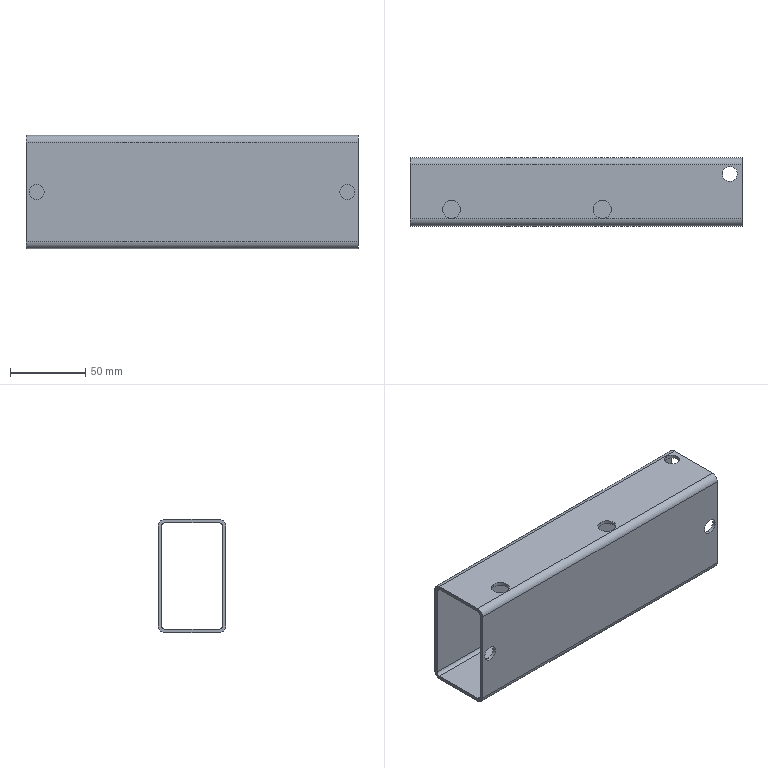Part | STEP file | [07] | 1 solid | 30 faces | box 220 x 45 x 75 mm | volume 112545 mm3 | cylinder 20 | plane 10 | commonest cylinder face diameters 10 x8 4.6 x4 9.2 x4 12 x4
STEP:
#1=CARTESIAN_POINT('',(213.,0.,32.5));
#2=VERTEX_POINT('',#1);
#3=CARTESIAN_POINT('',(213.,0.,42.5));
#4=VERTEX_POINT('',#3);
#5=CARTESIAN_POINT('',(213.,0.,37.5));
#6=DIRECTION('',(0.,1.,0.));
#7=DIRECTION('',(0.,0.,1.));
#8=AXIS2_PLACEMENT_3D('',#5,#6,#7);
#9=CIRCLE('',#8,5.);
#10=EDGE_CURVE('',#2,#4,#9,.T.);
#11=ORIENTED_EDGE('',*,*,#10,.F.);
#12=CARTESIAN_POINT('',(213.,2.3,32.5));
#13=VERTEX_POINT('',#12);
#14=CARTESIAN_POINT('',(213.,0.,32.5));
#15=DIRECTION('',(0.,1.,0.));
#16=VECTOR('',#15,1000.);
#17=LINE('',#14,#16);
#18=EDGE_CURVE('',#2,#13,#17,.T.);
#19=ORIENTED_EDGE('',*,*,#18,.T.);
#20=CARTESIAN_POINT('',(213.,2.3,42.5));
#21=VERTEX_POINT('',#20);
#22=CARTESIAN_POINT('',(213.,2.3,37.5));
#23=DIRECTION('',(0.,-1.,0.));
#24=DIRECTION('',(0.,0.,-1.));
#25=AXIS2_PLACEMENT_3D('',#22,#23,#24);
#26=CIRCLE('',#25,5.);
#27=EDGE_CURVE('',#21,#13,#26,.T.);
#28=ORIENTED_EDGE('',*,*,#27,.F.);
#29=CARTESIAN_POINT('',(213.,0.,42.5));
#30=DIRECTION('',(0.,1.,0.));
#31=VECTOR('',#30,1000.);
#32=LINE('',#29,#31);
#33=EDGE_CURVE('',#4,#21,#32,.T.);
#34=ORIENTED_EDGE('',*,*,#33,.F.);
#35=EDGE_LOOP('',(#11,#19,#28,#34));
#36=FACE_OUTER_BOUND('',#35,.T.);
#37=CARTESIAN_POINT('',(213.,0.,37.5));
#38=DIRECTION('',(0.,1.,0.));
#39=DIRECTION('',(0.,0.,1.));
#40=AXIS2_PLACEMENT_3D('',#37,#38,#39);
#41=CYLINDRICAL_SURFACE('',#40,5.);
#42=ADVANCED_FACE('',(#36),#41,.F.);
#43=CARTESIAN_POINT('',(7.,0.,32.5));
#44=VERTEX_POINT('',#43);
#45=CARTESIAN_POINT('',(7.,0.,42.5));
#46=VERTEX_POINT('',#45);
#47=CARTESIAN_POINT('',(7.,0.,37.5));
#48=DIRECTION('',(0.,1.,0.));
#49=DIRECTION('',(0.,0.,1.));
#50=AXIS2_PLACEMENT_3D('',#47,#48,#49);
#51=CIRCLE('',#50,5.);
#52=EDGE_CURVE('',#44,#46,#51,.T.);
#53=ORIENTED_EDGE('',*,*,#52,.F.);
#54=CARTESIAN_POINT('',(7.,2.3,32.5));
#55=VERTEX_POINT('',#54);
#56=CARTESIAN_POINT('',(7.,0.,32.5));
#57=DIRECTION('',(0.,1.,0.));
#58=VECTOR('',#57,1000.);
#59=LINE('',#56,#58);
#60=EDGE_CURVE('',#44,#55,#59,.T.);
#61=ORIENTED_EDGE('',*,*,#60,.T.);
#62=CARTESIAN_POINT('',(7.,2.3,42.5));
#63=VERTEX_POINT('',#62);
#64=CARTESIAN_POINT('',(7.,2.3,37.5));
#65=DIRECTION('',(0.,-1.,0.));
#66=DIRECTION('',(0.,0.,-1.));
#67=AXIS2_PLACEMENT_3D('',#64,#65,#66);
#68=CIRCLE('',#67,5.);
#69=EDGE_CURVE('',#63,#55,#68,.T.);
#70=ORIENTED_EDGE('',*,*,#69,.F.);
#71=CARTESIAN_POINT('',(7.,0.,42.5));
#72=DIRECTION('',(0.,1.,0.));
#73=VECTOR('',#72,1000.);
#74=LINE('',#71,#73);
#75=EDGE_CURVE('',#46,#63,#74,.T.);
#76=ORIENTED_EDGE('',*,*,#75,.F.);
#77=EDGE_LOOP('',(#53,#61,#70,#76));
#78=FACE_OUTER_BOUND('',#77,.T.);
#79=CARTESIAN_POINT('',(7.,0.,37.5));
#80=DIRECTION('',(0.,1.,0.));
#81=DIRECTION('',(0.,0.,1.));
#82=AXIS2_PLACEMENT_3D('',#79,#80,#81);
#83=CYLINDRICAL_SURFACE('',#82,5.);
#84=ADVANCED_FACE('',(#78),#83,.F.);
#85=CARTESIAN_POINT('',(212.,29.5,2.3));
#86=VERTEX_POINT('',#85);
#87=CARTESIAN_POINT('',(212.,39.5,2.3));
#88=VERTEX_POINT('',#87);
#89=CARTESIAN_POINT('',(212.,34.5,2.3));
#90=DIRECTION('',(0.,0.,-1.));
#91=DIRECTION('',(0.,1.,0.));
#92=AXIS2_PLACEMENT_3D('',#89,#90,#91);
#93=CIRCLE('',#92,5.);
#94=EDGE_CURVE('',#86,#88,#93,.T.);
#95=ORIENTED_EDGE('',*,*,#94,.F.);
#96=CARTESIAN_POINT('',(212.,29.5,0.));
#97=VERTEX_POINT('',#96);
#98=CARTESIAN_POINT('',(212.,29.5,2.3));
#99=DIRECTION('',(0.,0.,-1.));
#100=VECTOR('',#99,1000.);
#101=LINE('',#98,#100);
#102=EDGE_CURVE('',#86,#97,#101,.T.);
#103=ORIENTED_EDGE('',*,*,#102,.T.);
#104=CARTESIAN_POINT('',(212.,39.5,0.));
#105=VERTEX_POINT('',#104);
#106=CARTESIAN_POINT('',(212.,34.5,0.));
#107=DIRECTION('',(0.,0.,1.));
#108=DIRECTION('',(0.,-1.,0.));
#109=AXIS2_PLACEMENT_3D('',#106,#107,#108);
#110=CIRCLE('',#109,5.);
#111=EDGE_CURVE('',#105,#97,#110,.T.);
#112=ORIENTED_EDGE('',*,*,#111,.F.);
#113=CARTESIAN_POINT('',(212.,39.5,2.3));
#114=DIRECTION('',(0.,0.,-1.));
#115=VECTOR('',#114,1000.);
#116=LINE('',#113,#115);
#117=EDGE_CURVE('',#88,#105,#116,.T.);
#118=ORIENTED_EDGE('',*,*,#117,.F.);
#119=EDGE_LOOP('',(#95,#103,#112,#118));
#120=FACE_OUTER_BOUND('',#119,.T.);
#121=CARTESIAN_POINT('',(212.,34.5,2.3));
#122=DIRECTION('',(0.,0.,-1.));
#123=DIRECTION('',(0.,1.,0.));
#124=AXIS2_PLACEMENT_3D('',#121,#122,#123);
#125=CYLINDRICAL_SURFACE('',#124,5.);
#126=ADVANCED_FACE('',(#120),#125,.F.);
#127=CARTESIAN_POINT('',(127.5,5.,75.));
#128=VERTEX_POINT('',#127);
#129=CARTESIAN_POINT('',(127.5,17.,75.));
#130=VERTEX_POINT('',#129);
#131=CARTESIAN_POINT('',(127.5,11.,75.));
#132=DIRECTION('',(0.,0.,-1.));
#133=DIRECTION('',(0.,1.,0.));
#134=AXIS2_PLACEMENT_3D('',#131,#132,#133);
#135=CIRCLE('',#134,6.);
#136=EDGE_CURVE('',#128,#130,#135,.T.);
#137=ORIENTED_EDGE('',*,*,#136,.F.);
#138=CARTESIAN_POINT('',(127.5,5.,72.7));
#139=VERTEX_POINT('',#138);
#140=CARTESIAN_POINT('',(127.5,5.,75.));
#141=DIRECTION('',(0.,0.,-1.));
#142=VECTOR('',#141,1000.);
#143=LINE('',#140,#142);
#144=EDGE_CURVE('',#128,#139,#143,.T.);
#145=ORIENTED_EDGE('',*,*,#144,.T.);
#146=CARTESIAN_POINT('',(127.5,17.,72.7));
#147=VERTEX_POINT('',#146);
#148=CARTESIAN_POINT('',(127.5,11.,72.7));
#149=DIRECTION('',(0.,0.,1.));
#150=DIRECTION('',(0.,-1.,0.));
#151=AXIS2_PLACEMENT_3D('',#148,#149,#150);
#152=CIRCLE('',#151,6.);
#153=EDGE_CURVE('',#147,#139,#152,.T.);
#154=ORIENTED_EDGE('',*,*,#153,.F.);
#155=CARTESIAN_POINT('',(127.5,17.,75.));
#156=DIRECTION('',(0.,0.,-1.));
#157=VECTOR('',#156,1000.);
#158=LINE('',#155,#157);
#159=EDGE_CURVE('',#130,#147,#158,.T.);
#160=ORIENTED_EDGE('',*,*,#159,.F.);
#161=EDGE_LOOP('',(#137,#145,#154,#160));
#162=FACE_OUTER_BOUND('',#161,.T.);
#163=CARTESIAN_POINT('',(127.5,11.,75.));
#164=DIRECTION('',(0.,0.,-1.));
#165=DIRECTION('',(0.,1.,0.));
#166=AXIS2_PLACEMENT_3D('',#163,#164,#165);
#167=CYLINDRICAL_SURFACE('',#166,6.);
#168=ADVANCED_FACE('',(#162),#167,.F.);
#169=CARTESIAN_POINT('',(212.,29.5,75.));
#170=VERTEX_POINT('',#169);
#171=CARTESIAN_POINT('',(212.,39.5,75.));
#172=VERTEX_POINT('',#171);
#173=CARTESIAN_POINT('',(212.,34.5,75.));
#174=DIRECTION('',(0.,0.,-1.));
#175=DIRECTION('',(0.,1.,0.));
#176=AXIS2_PLACEMENT_3D('',#173,#174,#175);
#177=CIRCLE('',#176,5.);
#178=EDGE_CURVE('',#170,#172,#177,.T.);
#179=ORIENTED_EDGE('',*,*,#178,.F.);
#180=CARTESIAN_POINT('',(212.,29.5,72.7));
#181=VERTEX_POINT('',#180);
#182=CARTESIAN_POINT('',(212.,29.5,75.));
#183=DIRECTION('',(0.,0.,-1.));
#184=VECTOR('',#183,1000.);
#185=LINE('',#182,#184);
#186=EDGE_CURVE('',#170,#181,#185,.T.);
#187=ORIENTED_EDGE('',*,*,#186,.T.);
#188=CARTESIAN_POINT('',(212.,39.5,72.7));
#189=VERTEX_POINT('',#188);
#190=CARTESIAN_POINT('',(212.,34.5,72.7));
#191=DIRECTION('',(0.,0.,1.));
#192=DIRECTION('',(0.,-1.,0.));
#193=AXIS2_PLACEMENT_3D('',#190,#191,#192);
#194=CIRCLE('',#193,5.);
#195=EDGE_CURVE('',#189,#181,#194,.T.);
#196=ORIENTED_EDGE('',*,*,#195,.F.);
#197=CARTESIAN_POINT('',(212.,39.5,75.));
#198=DIRECTION('',(0.,0.,-1.));
#199=VECTOR('',#198,1000.);
#200=LINE('',#197,#199);
#201=EDGE_CURVE('',#172,#189,#200,.T.);
#202=ORIENTED_EDGE('',*,*,#201,.F.);
#203=EDGE_LOOP('',(#179,#187,#196,#202));
#204=FACE_OUTER_BOUND('',#203,.T.);
#205=CARTESIAN_POINT('',(212.,34.5,75.));
#206=DIRECTION('',(0.,0.,-1.));
#207=DIRECTION('',(0.,1.,0.));
#208=AXIS2_PLACEMENT_3D('',#205,#206,#207);
#209=CYLINDRICAL_SURFACE('',#208,5.);
#210=ADVANCED_FACE('',(#204),#209,.F.);
#211=CARTESIAN_POINT('',(27.5,5.,75.));
#212=VERTEX_POINT('',#211);
#213=CARTESIAN_POINT('',(27.5,17.,75.));
#214=VERTEX_POINT('',#213);
#215=CARTESIAN_POINT('',(27.5,11.,75.));
#216=DIRECTION('',(0.,0.,-1.));
#217=DIRECTION('',(0.,1.,0.));
#218=AXIS2_PLACEMENT_3D('',#215,#216,#217);
#219=CIRCLE('',#218,6.);
#220=EDGE_CURVE('',#212,#214,#219,.T.);
#221=ORIENTED_EDGE('',*,*,#220,.F.);
#222=CARTESIAN_POINT('',(27.5,5.,72.7));
#223=VERTEX_POINT('',#222);
#224=CARTESIAN_POINT('',(27.5,5.,75.));
#225=DIRECTION('',(0.,0.,-1.));
#226=VECTOR('',#225,1000.);
#227=LINE('',#224,#226);
#228=EDGE_CURVE('',#212,#223,#227,.T.);
#229=ORIENTED_EDGE('',*,*,#228,.T.);
#230=CARTESIAN_POINT('',(27.5,17.,72.7));
#231=VERTEX_POINT('',#230);
#232=CARTESIAN_POINT('',(27.5,11.,72.7));
#233=DIRECTION('',(0.,0.,1.));
#234=DIRECTION('',(0.,-1.,0.));
#235=AXIS2_PLACEMENT_3D('',#232,#233,#234);
#236=CIRCLE('',#235,6.);
#237=EDGE_CURVE('',#231,#223,#236,.T.);
#238=ORIENTED_EDGE('',*,*,#237,.F.);
#239=CARTESIAN_POINT('',(27.5,17.,75.));
#240=DIRECTION('',(0.,0.,-1.));
#241=VECTOR('',#240,1000.);
#242=LINE('',#239,#241);
#243=EDGE_CURVE('',#214,#231,#242,.T.);
#244=ORIENTED_EDGE('',*,*,#243,.F.);
#245=EDGE_LOOP('',(#221,#229,#238,#244));
#246=FACE_OUTER_BOUND('',#245,.T.);
#247=CARTESIAN_POINT('',(27.5,11.,75.));
#248=DIRECTION('',(0.,0.,-1.));
#249=DIRECTION('',(0.,1.,0.));
#250=AXIS2_PLACEMENT_3D('',#247,#248,#249);
#251=CYLINDRICAL_SURFACE('',#250,6.);
#252=ADVANCED_FACE('',(#246),#251,.F.);
#253=CARTESIAN_POINT('',(213.,0.,37.5));
#254=DIRECTION('',(0.,1.,0.));
#255=DIRECTION('',(0.,0.,1.));
#256=AXIS2_PLACEMENT_3D('',#253,#254,#255);
#257=CIRCLE('',#256,5.);
#258=EDGE_CURVE('',#4,#2,#257,.T.);
#259=ORIENTED_EDGE('',*,*,#258,.T.);
#260=ORIENTED_EDGE('',*,*,#10,.T.);
#261=EDGE_LOOP('',(#259,#260));
#262=FACE_BOUND('',#261,.T.);
#263=CARTESIAN_POINT('',(7.,0.,37.5));
#264=DIRECTION('',(0.,1.,0.));
#265=DIRECTION('',(0.,0.,1.));
#266=AXIS2_PLACEMENT_3D('',#263,#264,#265);
#267=CIRCLE('',#266,5.);
#268=EDGE_CURVE('',#46,#44,#267,.T.);
#269=ORIENTED_EDGE('',*,*,#268,.T.);
#270=ORIENTED_EDGE('',*,*,#52,.T.);
#271=EDGE_LOOP('',(#269,#270));
#272=FACE_BOUND('',#271,.T.);
#273=CARTESIAN_POINT('',(220.,0.,70.4));
#274=VERTEX_POINT('',#273);
#275=CARTESIAN_POINT('',(220.,0.,4.6));
#276=VERTEX_POINT('',#275);
#277=CARTESIAN_POINT('',(220.,0.,70.4));
#278=DIRECTION('',(0.,0.,-1.));
#279=VECTOR('',#278,1000.);
#280=LINE('',#277,#279);
#281=EDGE_CURVE('',#274,#276,#280,.T.);
#282=ORIENTED_EDGE('',*,*,#281,.F.);
#283=CARTESIAN_POINT('',(0.,0.,70.4));
#284=VERTEX_POINT('',#283);
#285=CARTESIAN_POINT('',(0.,0.,70.4));
#286=DIRECTION('',(1.,0.,0.));
#287=VECTOR('',#286,1000.);
#288=LINE('',#285,#287);
#289=EDGE_CURVE('',#284,#274,#288,.T.);
#290=ORIENTED_EDGE('',*,*,#289,.F.);
#291=CARTESIAN_POINT('',(0.,0.,4.6));
#292=VERTEX_POINT('',#291);
#293=CARTESIAN_POINT('',(0.,0.,70.4));
#294=DIRECTION('',(0.,0.,-1.));
#295=VECTOR('',#294,1000.);
#296=LINE('',#293,#295);
#297=EDGE_CURVE('',#284,#292,#296,.T.);
#298=ORIENTED_EDGE('',*,*,#297,.T.);
#299=CARTESIAN_POINT('',(0.,0.,4.6));
#300=DIRECTION('',(1.,0.,0.));
#301=VECTOR('',#300,1000.);
#302=LINE('',#299,#301);
#303=EDGE_CURVE('',#292,#276,#302,.T.);
#304=ORIENTED_EDGE('',*,*,#303,.T.);
#305=EDGE_LOOP('',(#282,#290,#298,#304));
#306=FACE_OUTER_BOUND('',#305,.T.);
#307=CARTESIAN_POINT('',(0.,0.,70.4));
#308=DIRECTION('',(0.,-1.,0.));
#309=DIRECTION('',(0.,0.,-1.));
#310=AXIS2_PLACEMENT_3D('',#307,#308,#309);
#311=PLANE('',#310);
#312=ADVANCED_FACE('',(#262,#272,#306),#311,.T.);
#313=CARTESIAN_POINT('',(220.,4.6,0.));
#314=VERTEX_POINT('',#313);
#315=CARTESIAN_POINT('',(220.,4.6,4.6));
#316=DIRECTION('',(1.,0.,0.));
#317=DIRECTION('',(0.,-1.,0.));
#318=AXIS2_PLACEMENT_3D('',#315,#316,#317);
#319=CIRCLE('',#318,4.6);
#320=EDGE_CURVE('',#276,#314,#319,.T.);
#321=ORIENTED_EDGE('',*,*,#320,.F.);
#322=ORIENTED_EDGE('',*,*,#303,.F.);
#323=CARTESIAN_POINT('',(0.,4.6,0.));
#324=VERTEX_POINT('',#323);
#325=CARTESIAN_POINT('',(0.,4.6,4.6));
#326=DIRECTION('',(1.,0.,0.));
#327=DIRECTION('',(0.,-1.,0.));
#328=AXIS2_PLACEMENT_3D('',#325,#326,#327);
#329=CIRCLE('',#328,4.6);
#330=EDGE_CURVE('',#292,#324,#329,.T.);
#331=ORIENTED_EDGE('',*,*,#330,.T.);
#332=CARTESIAN_POINT('',(0.,4.6,0.));
#333=DIRECTION('',(1.,0.,0.));
#334=VECTOR('',#333,1000.);
#335=LINE('',#332,#334);
#336=EDGE_CURVE('',#324,#314,#335,.T.);
#337=ORIENTED_EDGE('',*,*,#336,.T.);
#338=EDGE_LOOP('',(#321,#322,#331,#337));
#339=FACE_OUTER_BOUND('',#338,.T.);
#340=CARTESIAN_POINT('',(0.,4.6,4.6));
#341=DIRECTION('',(1.,0.,0.));
#342=DIRECTION('',(0.,-1.,0.));
#343=AXIS2_PLACEMENT_3D('',#340,#341,#342);
#344=CYLINDRICAL_SURFACE('',#343,4.6);
#345=ADVANCED_FACE('',(#339),#344,.T.);
#346=ORIENTED_EDGE('',*,*,#111,.T.);
#347=CARTESIAN_POINT('',(212.,34.5,0.));
#348=DIRECTION('',(0.,0.,1.));
#349=DIRECTION('',(0.,-1.,0.));
#350=AXIS2_PLACEMENT_3D('',#347,#348,#349);
#351=CIRCLE('',#350,5.);
#352=EDGE_CURVE('',#97,#105,#351,.T.);
#353=ORIENTED_EDGE('',*,*,#352,.T.);
#354=EDGE_LOOP('',(#346,#353));
#355=FACE_BOUND('',#354,.T.);
#356=CARTESIAN_POINT('',(220.,40.4,0.));
#357=VERTEX_POINT('',#356);
#358=CARTESIAN_POINT('',(220.,4.6,0.));
#359=DIRECTION('',(0.,1.,0.));
#360=VECTOR('',#359,1000.);
#361=LINE('',#358,#360);
#362=EDGE_CURVE('',#314,#357,#361,.T.);
#363=ORIENTED_EDGE('',*,*,#362,.F.);
#364=ORIENTED_EDGE('',*,*,#336,.F.);
#365=CARTESIAN_POINT('',(0.,40.4,0.));
#366=VERTEX_POINT('',#365);
#367=CARTESIAN_POINT('',(0.,4.6,0.));
#368=DIRECTION('',(0.,1.,0.));
#369=VECTOR('',#368,1000.);
#370=LINE('',#367,#369);
#371=EDGE_CURVE('',#324,#366,#370,.T.);
#372=ORIENTED_EDGE('',*,*,#371,.T.);
#373=CARTESIAN_POINT('',(0.,40.4,0.));
#374=DIRECTION('',(1.,0.,0.));
#375=VECTOR('',#374,1000.);
#376=LINE('',#373,#375);
#377=EDGE_CURVE('',#366,#357,#376,.T.);
#378=ORIENTED_EDGE('',*,*,#377,.T.);
#379=EDGE_LOOP('',(#363,#364,#372,#378));
#380=FACE_OUTER_BOUND('',#379,.T.);
#381=CARTESIAN_POINT('',(0.,4.6,0.));
#382=DIRECTION('',(0.,0.,-1.));
#383=DIRECTION('',(0.,1.,0.));
#384=AXIS2_PLACEMENT_3D('',#381,#382,#383);
#385=PLANE('',#384);
#386=ADVANCED_FACE('',(#355,#380),#385,.T.);
#387=CARTESIAN_POINT('',(220.,45.,4.6));
#388=VERTEX_POINT('',#387);
#389=CARTESIAN_POINT('',(220.,40.4,4.6));
#390=DIRECTION('',(1.,0.,0.));
#391=DIRECTION('',(0.,-1.,0.));
#392=AXIS2_PLACEMENT_3D('',#389,#390,#391);
#393=CIRCLE('',#392,4.6);
#394=EDGE_CURVE('',#357,#388,#393,.T.);
#395=ORIENTED_EDGE('',*,*,#394,.F.);
#396=ORIENTED_EDGE('',*,*,#377,.F.);
#397=CARTESIAN_POINT('',(0.,45.,4.6));
#398=VERTEX_POINT('',#397);
#399=CARTESIAN_POINT('',(0.,40.4,4.6));
#400=DIRECTION('',(1.,0.,0.));
#401=DIRECTION('',(0.,-1.,0.));
#402=AXIS2_PLACEMENT_3D('',#399,#400,#401);
#403=CIRCLE('',#402,4.6);
#404=EDGE_CURVE('',#366,#398,#403,.T.);
#405=ORIENTED_EDGE('',*,*,#404,.T.);
#406=CARTESIAN_POINT('',(0.,45.,4.6));
#407=DIRECTION('',(1.,0.,0.));
#408=VECTOR('',#407,1000.);
#409=LINE('',#406,#408);
#410=EDGE_CURVE('',#398,#388,#409,.T.);
#411=ORIENTED_EDGE('',*,*,#410,.T.);
#412=EDGE_LOOP('',(#395,#396,#405,#411));
#413=FACE_OUTER_BOUND('',#412,.T.);
#414=CARTESIAN_POINT('',(0.,40.4,4.6));
#415=DIRECTION('',(1.,0.,0.));
#416=DIRECTION('',(0.,-1.,0.));
#417=AXIS2_PLACEMENT_3D('',#414,#415,#416);
#418=CYLINDRICAL_SURFACE('',#417,4.6);
#419=ADVANCED_FACE('',(#413),#418,.T.);
#420=CARTESIAN_POINT('',(220.,45.,70.4));
#421=VERTEX_POINT('',#420);
#422=CARTESIAN_POINT('',(220.,45.,4.6));
#423=DIRECTION('',(0.,0.,1.));
#424=VECTOR('',#423,1000.);
#425=LINE('',#422,#424);
#426=EDGE_CURVE('',#388,#421,#425,.T.);
#427=ORIENTED_EDGE('',*,*,#426,.F.);
#428=ORIENTED_EDGE('',*,*,#410,.F.);
#429=CARTESIAN_POINT('',(0.,45.,70.4));
#430=VERTEX_POINT('',#429);
#431=CARTESIAN_POINT('',(0.,45.,4.6));
#432=DIRECTION('',(0.,0.,1.));
#433=VECTOR('',#432,1000.);
#434=LINE('',#431,#433);
#435=EDGE_CURVE('',#398,#430,#434,.T.);
#436=ORIENTED_EDGE('',*,*,#435,.T.);
#437=CARTESIAN_POINT('',(0.,45.,70.4));
#438=DIRECTION('',(1.,0.,0.));
#439=VECTOR('',#438,1000.);
#440=LINE('',#437,#439);
#441=EDGE_CURVE('',#430,#421,#440,.T.);
#442=ORIENTED_EDGE('',*,*,#441,.T.);
#443=EDGE_LOOP('',(#427,#428,#436,#442));
#444=FACE_OUTER_BOUND('',#443,.T.);
#445=CARTESIAN_POINT('',(0.,45.,4.6));
#446=DIRECTION('',(0.,1.,0.));
#447=DIRECTION('',(0.,0.,1.));
#448=AXIS2_PLACEMENT_3D('',#445,#446,#447);
#449=PLANE('',#448);
#450=ADVANCED_FACE('',(#444),#449,.T.);
#451=CARTESIAN_POINT('',(220.,40.4,75.));
#452=VERTEX_POINT('',#451);
#453=CARTESIAN_POINT('',(220.,40.4,70.4));
#454=DIRECTION('',(1.,0.,0.));
#455=DIRECTION('',(0.,-1.,0.));
#456=AXIS2_PLACEMENT_3D('',#453,#454,#455);
#457=CIRCLE('',#456,4.6);
#458=EDGE_CURVE('',#421,#452,#457,.T.);
#459=ORIENTED_EDGE('',*,*,#458,.F.);
#460=ORIENTED_EDGE('',*,*,#441,.F.);
#461=CARTESIAN_POINT('',(0.,40.4,75.));
#462=VERTEX_POINT('',#461);
#463=CARTESIAN_POINT('',(0.,40.4,70.4));
#464=DIRECTION('',(1.,0.,0.));
#465=DIRECTION('',(0.,-1.,0.));
#466=AXIS2_PLACEMENT_3D('',#463,#464,#465);
#467=CIRCLE('',#466,4.6);
#468=EDGE_CURVE('',#430,#462,#467,.T.);
#469=ORIENTED_EDGE('',*,*,#468,.T.);
#470=CARTESIAN_POINT('',(0.,40.4,75.));
#471=DIRECTION('',(1.,0.,0.));
#472=VECTOR('',#471,1000.);
#473=LINE('',#470,#472);
#474=EDGE_CURVE('',#462,#452,#473,.T.);
#475=ORIENTED_EDGE('',*,*,#474,.T.);
#476=EDGE_LOOP('',(#459,#460,#469,#475));
#477=FACE_OUTER_BOUND('',#476,.T.);
#478=CARTESIAN_POINT('',(0.,40.4,70.4));
#479=DIRECTION('',(1.,0.,0.));
#480=DIRECTION('',(0.,-1.,0.));
#481=AXIS2_PLACEMENT_3D('',#478,#479,#480);
#482=CYLINDRICAL_SURFACE('',#481,4.6);
#483=ADVANCED_FACE('',(#477),#482,.T.);
#484=CARTESIAN_POINT('',(127.5,11.,75.));
#485=DIRECTION('',(0.,0.,-1.));
#486=DIRECTION('',(0.,1.,0.));
#487=AXIS2_PLACEMENT_3D('',#484,#485,#486);
#488=CIRCLE('',#487,6.);
#489=EDGE_CURVE('',#130,#128,#488,.T.);
#490=ORIENTED_EDGE('',*,*,#489,.T.);
#491=ORIENTED_EDGE('',*,*,#136,.T.);
#492=EDGE_LOOP('',(#490,#491));
#493=FACE_BOUND('',#492,.T.);
#494=CARTESIAN_POINT('',(212.,34.5,75.));
#495=DIRECTION('',(0.,0.,-1.));
#496=DIRECTION('',(0.,1.,0.));
#497=AXIS2_PLACEMENT_3D('',#494,#495,#496);
#498=CIRCLE('',#497,5.);
#499=EDGE_CURVE('',#172,#170,#498,.T.);
#500=ORIENTED_EDGE('',*,*,#499,.T.);
#501=ORIENTED_EDGE('',*,*,#178,.T.);
#502=EDGE_LOOP('',(#500,#501));
#503=FACE_BOUND('',#502,.T.);
#504=CARTESIAN_POINT('',(27.5,11.,75.));
#505=DIRECTION('',(0.,0.,-1.));
#506=DIRECTION('',(0.,1.,0.));
#507=AXIS2_PLACEMENT_3D('',#504,#505,#506);
#508=CIRCLE('',#507,6.);
#509=EDGE_CURVE('',#214,#212,#508,.T.);
#510=ORIENTED_EDGE('',*,*,#509,.T.);
#511=ORIENTED_EDGE('',*,*,#220,.T.);
#512=EDGE_LOOP('',(#510,#511));
#513=FACE_BOUND('',#512,.T.);
#514=CARTESIAN_POINT('',(220.,4.6,75.));
#515=VERTEX_POINT('',#514);
#516=CARTESIAN_POINT('',(220.,40.4,75.));
#517=DIRECTION('',(0.,-1.,0.));
#518=VECTOR('',#517,1000.);
#519=LINE('',#516,#518);
#520=EDGE_CURVE('',#452,#515,#519,.T.);
#521=ORIENTED_EDGE('',*,*,#520,.F.);
#522=ORIENTED_EDGE('',*,*,#474,.F.);
#523=CARTESIAN_POINT('',(0.,4.6,75.));
#524=VERTEX_POINT('',#523);
#525=CARTESIAN_POINT('',(0.,40.4,75.));
#526=DIRECTION('',(0.,-1.,0.));
#527=VECTOR('',#526,1000.);
#528=LINE('',#525,#527);
#529=EDGE_CURVE('',#462,#524,#528,.T.);
#530=ORIENTED_EDGE('',*,*,#529,.T.);
#531=CARTESIAN_POINT('',(0.,4.6,75.));
#532=DIRECTION('',(1.,0.,0.));
#533=VECTOR('',#532,1000.);
#534=LINE('',#531,#533);
#535=EDGE_CURVE('',#524,#515,#534,.T.);
#536=ORIENTED_EDGE('',*,*,#535,.T.);
#537=EDGE_LOOP('',(#521,#522,#530,#536));
#538=FACE_OUTER_BOUND('',#537,.T.);
#539=CARTESIAN_POINT('',(0.,40.4,75.));
#540=DIRECTION('',(0.,0.,1.));
#541=DIRECTION('',(-1.,0.,0.));
#542=AXIS2_PLACEMENT_3D('',#539,#540,#541);
#543=PLANE('',#542);
#544=ADVANCED_FACE('',(#493,#503,#513,#538),#543,.T.);
#545=CARTESIAN_POINT('',(220.,4.6,70.4));
#546=DIRECTION('',(1.,0.,0.));
#547=DIRECTION('',(0.,-1.,0.));
#548=AXIS2_PLACEMENT_3D('',#545,#546,#547);
#549=CIRCLE('',#548,4.6);
#550=EDGE_CURVE('',#515,#274,#549,.T.);
#551=ORIENTED_EDGE('',*,*,#550,.F.);
#552=ORIENTED_EDGE('',*,*,#535,.F.);
#553=CARTESIAN_POINT('',(0.,4.6,70.4));
#554=DIRECTION('',(1.,0.,0.));
#555=DIRECTION('',(0.,-1.,0.));
#556=AXIS2_PLACEMENT_3D('',#553,#554,#555);
#557=CIRCLE('',#556,4.6);
#558=EDGE_CURVE('',#524,#284,#557,.T.);
#559=ORIENTED_EDGE('',*,*,#558,.T.);
#560=ORIENTED_EDGE('',*,*,#289,.T.);
#561=EDGE_LOOP('',(#551,#552,#559,#560));
#562=FACE_OUTER_BOUND('',#561,.T.);
#563=CARTESIAN_POINT('',(0.,4.6,70.4));
#564=DIRECTION('',(1.,0.,0.));
#565=DIRECTION('',(0.,-1.,0.));
#566=AXIS2_PLACEMENT_3D('',#563,#564,#565);
#567=CYLINDRICAL_SURFACE('',#566,4.6);
#568=ADVANCED_FACE('',(#562),#567,.T.);
#569=CARTESIAN_POINT('',(0.,40.4,72.7));
#570=VERTEX_POINT('',#569);
#571=CARTESIAN_POINT('',(0.,4.6,72.7));
#572=VERTEX_POINT('',#571);
#573=CARTESIAN_POINT('',(0.,40.4,72.7));
#574=DIRECTION('',(0.,-1.,0.));
#575=VECTOR('',#574,1000.);
#576=LINE('',#573,#575);
#577=EDGE_CURVE('',#570,#572,#576,.T.);
#578=ORIENTED_EDGE('',*,*,#577,.T.);
#579=CARTESIAN_POINT('',(0.,2.3,70.4));
#580=VERTEX_POINT('',#579);
#581=CARTESIAN_POINT('',(0.,4.6,70.4));
#582=DIRECTION('',(1.,0.,0.));
#583=DIRECTION('',(0.,0.,1.));
#584=AXIS2_PLACEMENT_3D('',#581,#582,#583);
#585=CIRCLE('',#584,2.3);
#586=EDGE_CURVE('',#572,#580,#585,.T.);
#587=ORIENTED_EDGE('',*,*,#586,.T.);
#588=CARTESIAN_POINT('',(0.,2.3,4.6));
#589=VERTEX_POINT('',#588);
#590=CARTESIAN_POINT('',(0.,2.3,70.4));
#591=DIRECTION('',(0.,0.,-1.));
#592=VECTOR('',#591,1000.);
#593=LINE('',#590,#592);
#594=EDGE_CURVE('',#580,#589,#593,.T.);
#595=ORIENTED_EDGE('',*,*,#594,.T.);
#596=CARTESIAN_POINT('',(0.,4.6,2.3));
#597=VERTEX_POINT('',#596);
#598=CARTESIAN_POINT('',(0.,4.6,4.6));
#599=DIRECTION('',(1.,0.,0.));
#600=DIRECTION('',(0.,0.,1.));
#601=AXIS2_PLACEMENT_3D('',#598,#599,#600);
#602=CIRCLE('',#601,2.3);
#603=EDGE_CURVE('',#589,#597,#602,.T.);
#604=ORIENTED_EDGE('',*,*,#603,.T.);
#605=CARTESIAN_POINT('',(0.,40.4,2.3));
#606=VERTEX_POINT('',#605);
#607=CARTESIAN_POINT('',(0.,4.6,2.3));
#608=DIRECTION('',(0.,1.,0.));
#609=VECTOR('',#608,1000.);
#610=LINE('',#607,#609);
#611=EDGE_CURVE('',#597,#606,#610,.T.);
#612=ORIENTED_EDGE('',*,*,#611,.T.);
#613=CARTESIAN_POINT('',(0.,42.7,4.6));
#614=VERTEX_POINT('',#613);
#615=CARTESIAN_POINT('',(0.,40.4,4.6));
#616=DIRECTION('',(1.,0.,0.));
#617=DIRECTION('',(0.,0.,1.));
#618=AXIS2_PLACEMENT_3D('',#615,#616,#617);
#619=CIRCLE('',#618,2.3);
#620=EDGE_CURVE('',#606,#614,#619,.T.);
#621=ORIENTED_EDGE('',*,*,#620,.T.);
#622=CARTESIAN_POINT('',(0.,42.7,70.4));
#623=VERTEX_POINT('',#622);
#624=CARTESIAN_POINT('',(0.,42.7,4.6));
#625=DIRECTION('',(0.,0.,1.));
#626=VECTOR('',#625,1000.);
#627=LINE('',#624,#626);
#628=EDGE_CURVE('',#614,#623,#627,.T.);
#629=ORIENTED_EDGE('',*,*,#628,.T.);
#630=CARTESIAN_POINT('',(0.,40.4,70.4));
#631=DIRECTION('',(1.,0.,0.));
#632=DIRECTION('',(0.,0.,1.));
#633=AXIS2_PLACEMENT_3D('',#630,#631,#632);
#634=CIRCLE('',#633,2.3);
#635=EDGE_CURVE('',#623,#570,#634,.T.);
#636=ORIENTED_EDGE('',*,*,#635,.T.);
#637=EDGE_LOOP('',(#578,#587,#595,#604,#612,#621,#629,#636));
#638=FACE_BOUND('',#637,.T.);
#639=ORIENTED_EDGE('',*,*,#297,.F.);
#640=ORIENTED_EDGE('',*,*,#558,.F.);
#641=ORIENTED_EDGE('',*,*,#529,.F.);
#642=ORIENTED_EDGE('',*,*,#468,.F.);
#643=ORIENTED_EDGE('',*,*,#435,.F.);
#644=ORIENTED_EDGE('',*,*,#404,.F.);
#645=ORIENTED_EDGE('',*,*,#371,.F.);
#646=ORIENTED_EDGE('',*,*,#330,.F.);
#647=EDGE_LOOP('',(#639,#640,#641,#642,#643,#644,#645,#646));
#648=FACE_OUTER_BOUND('',#647,.T.);
#649=CARTESIAN_POINT('',(0.,4.6,4.6));
#650=DIRECTION('',(1.,0.,0.));
#651=DIRECTION('',(0.,-1.,0.));
#652=AXIS2_PLACEMENT_3D('',#649,#650,#651);
#653=PLANE('',#652);
#654=ADVANCED_FACE('',(#638,#648),#653,.F.);
#655=CARTESIAN_POINT('',(220.,4.6,72.7));
#656=VERTEX_POINT('',#655);
#657=CARTESIAN_POINT('',(220.,2.3,70.4));
#658=VERTEX_POINT('',#657);
#659=CARTESIAN_POINT('',(220.,4.6,70.4));
#660=DIRECTION('',(1.,0.,0.));
#661=DIRECTION('',(0.,0.,1.));
#662=AXIS2_PLACEMENT_3D('',#659,#660,#661);
#663=CIRCLE('',#662,2.3);
#664=EDGE_CURVE('',#656,#658,#663,.T.);
#665=ORIENTED_EDGE('',*,*,#664,.F.);
#666=CARTESIAN_POINT('',(220.,40.4,72.7));
#667=VERTEX_POINT('',#666);
#668=CARTESIAN_POINT('',(220.,40.4,72.7));
#669=DIRECTION('',(0.,-1.,0.));
#670=VECTOR('',#669,1000.);
#671=LINE('',#668,#670);
#672=EDGE_CURVE('',#667,#656,#671,.T.);
#673=ORIENTED_EDGE('',*,*,#672,.F.);
#674=CARTESIAN_POINT('',(220.,42.7,70.4));
#675=VERTEX_POINT('',#674);
#676=CARTESIAN_POINT('',(220.,40.4,70.4));
#677=DIRECTION('',(1.,0.,0.));
#678=DIRECTION('',(0.,0.,1.));
#679=AXIS2_PLACEMENT_3D('',#676,#677,#678);
#680=CIRCLE('',#679,2.3);
#681=EDGE_CURVE('',#675,#667,#680,.T.);
#682=ORIENTED_EDGE('',*,*,#681,.F.);
#683=CARTESIAN_POINT('',(220.,42.7,4.6));
#684=VERTEX_POINT('',#683);
#685=CARTESIAN_POINT('',(220.,42.7,4.6));
#686=DIRECTION('',(0.,0.,1.));
#687=VECTOR('',#686,1000.);
#688=LINE('',#685,#687);
#689=EDGE_CURVE('',#684,#675,#688,.T.);
#690=ORIENTED_EDGE('',*,*,#689,.F.);
#691=CARTESIAN_POINT('',(220.,40.4,2.3));
#692=VERTEX_POINT('',#691);
#693=CARTESIAN_POINT('',(220.,40.4,4.6));
#694=DIRECTION('',(1.,0.,0.));
#695=DIRECTION('',(0.,0.,1.));
#696=AXIS2_PLACEMENT_3D('',#693,#694,#695);
#697=CIRCLE('',#696,2.3);
#698=EDGE_CURVE('',#692,#684,#697,.T.);
#699=ORIENTED_EDGE('',*,*,#698,.F.);
#700=CARTESIAN_POINT('',(220.,4.6,2.3));
#701=VERTEX_POINT('',#700);
#702=CARTESIAN_POINT('',(220.,4.6,2.3));
#703=DIRECTION('',(0.,1.,0.));
#704=VECTOR('',#703,1000.);
#705=LINE('',#702,#704);
#706=EDGE_CURVE('',#701,#692,#705,.T.);
#707=ORIENTED_EDGE('',*,*,#706,.F.);
#708=CARTESIAN_POINT('',(220.,2.3,4.6));
#709=VERTEX_POINT('',#708);
#710=CARTESIAN_POINT('',(220.,4.6,4.6));
#711=DIRECTION('',(1.,0.,0.));
#712=DIRECTION('',(0.,0.,1.));
#713=AXIS2_PLACEMENT_3D('',#710,#711,#712);
#714=CIRCLE('',#713,2.3);
#715=EDGE_CURVE('',#709,#701,#714,.T.);
#716=ORIENTED_EDGE('',*,*,#715,.F.);
#717=CARTESIAN_POINT('',(220.,2.3,70.4));
#718=DIRECTION('',(0.,0.,-1.));
#719=VECTOR('',#718,1000.);
#720=LINE('',#717,#719);
#721=EDGE_CURVE('',#658,#709,#720,.T.);
#722=ORIENTED_EDGE('',*,*,#721,.F.);
#723=EDGE_LOOP('',(#665,#673,#682,#690,#699,#707,#716,#722));
#724=FACE_BOUND('',#723,.T.);
#725=ORIENTED_EDGE('',*,*,#281,.T.);
#726=ORIENTED_EDGE('',*,*,#320,.T.);
#727=ORIENTED_EDGE('',*,*,#362,.T.);
#728=ORIENTED_EDGE('',*,*,#394,.T.);
#729=ORIENTED_EDGE('',*,*,#426,.T.);
#730=ORIENTED_EDGE('',*,*,#458,.T.);
#731=ORIENTED_EDGE('',*,*,#520,.T.);
#732=ORIENTED_EDGE('',*,*,#550,.T.);
#733=EDGE_LOOP('',(#725,#726,#727,#728,#729,#730,#731,#732));
#734=FACE_OUTER_BOUND('',#733,.T.);
#735=CARTESIAN_POINT('',(220.,4.6,4.6));
#736=DIRECTION('',(1.,0.,0.));
#737=DIRECTION('',(0.,-1.,0.));
#738=AXIS2_PLACEMENT_3D('',#735,#736,#737);
#739=PLANE('',#738);
#740=ADVANCED_FACE('',(#724,#734),#739,.T.);
#741=ORIENTED_EDGE('',*,*,#664,.T.);
#742=CARTESIAN_POINT('',(0.,2.3,70.4));
#743=DIRECTION('',(1.,0.,0.));
#744=VECTOR('',#743,1000.);
#745=LINE('',#742,#744);
#746=EDGE_CURVE('',#580,#658,#745,.T.);
#747=ORIENTED_EDGE('',*,*,#746,.F.);
#748=ORIENTED_EDGE('',*,*,#586,.F.);
#749=CARTESIAN_POINT('',(0.,4.6,72.7));
#750=DIRECTION('',(1.,0.,0.));
#751=VECTOR('',#750,1000.);
#752=LINE('',#749,#751);
#753=EDGE_CURVE('',#572,#656,#752,.T.);
#754=ORIENTED_EDGE('',*,*,#753,.T.);
#755=EDGE_LOOP('',(#741,#747,#748,#754));
#756=FACE_OUTER_BOUND('',#755,.T.);
#757=CARTESIAN_POINT('',(0.,4.6,70.4));
#758=DIRECTION('',(1.,0.,0.));
#759=DIRECTION('',(0.,0.,1.));
#760=AXIS2_PLACEMENT_3D('',#757,#758,#759);
#761=CYLINDRICAL_SURFACE('',#760,2.3);
#762=ADVANCED_FACE('',(#756),#761,.F.);
#763=ORIENTED_EDGE('',*,*,#27,.T.);
#764=CARTESIAN_POINT('',(213.,2.3,37.5));
#765=DIRECTION('',(0.,-1.,0.));
#766=DIRECTION('',(0.,0.,-1.));
#767=AXIS2_PLACEMENT_3D('',#764,#765,#766);
#768=CIRCLE('',#767,5.);
#769=EDGE_CURVE('',#13,#21,#768,.T.);
#770=ORIENTED_EDGE('',*,*,#769,.T.);
#771=EDGE_LOOP('',(#763,#770));
#772=FACE_BOUND('',#771,.T.);
#773=ORIENTED_EDGE('',*,*,#69,.T.);
#774=CARTESIAN_POINT('',(7.,2.3,37.5));
#775=DIRECTION('',(0.,-1.,0.));
#776=DIRECTION('',(0.,0.,-1.));
#777=AXIS2_PLACEMENT_3D('',#774,#775,#776);
#778=CIRCLE('',#777,5.);
#779=EDGE_CURVE('',#55,#63,#778,.T.);
#780=ORIENTED_EDGE('',*,*,#779,.T.);
#781=EDGE_LOOP('',(#773,#780));
#782=FACE_BOUND('',#781,.T.);
#783=ORIENTED_EDGE('',*,*,#721,.T.);
#784=CARTESIAN_POINT('',(0.,2.3,4.6));
#785=DIRECTION('',(1.,0.,0.));
#786=VECTOR('',#785,1000.);
#787=LINE('',#784,#786);
#788=EDGE_CURVE('',#589,#709,#787,.T.);
#789=ORIENTED_EDGE('',*,*,#788,.F.);
#790=ORIENTED_EDGE('',*,*,#594,.F.);
#791=ORIENTED_EDGE('',*,*,#746,.T.);
#792=EDGE_LOOP('',(#783,#789,#790,#791));
#793=FACE_OUTER_BOUND('',#792,.T.);
#794=CARTESIAN_POINT('',(0.,2.3,70.4));
#795=DIRECTION('',(0.,-1.,0.));
#796=DIRECTION('',(1.,0.,0.));
#797=AXIS2_PLACEMENT_3D('',#794,#795,#796);
#798=PLANE('',#797);
#799=ADVANCED_FACE('',(#772,#782,#793),#798,.F.);
#800=ORIENTED_EDGE('',*,*,#715,.T.);
#801=CARTESIAN_POINT('',(0.,4.6,2.3));
#802=DIRECTION('',(1.,0.,0.));
#803=VECTOR('',#802,1000.);
#804=LINE('',#801,#803);
#805=EDGE_CURVE('',#597,#701,#804,.T.);
#806=ORIENTED_EDGE('',*,*,#805,.F.);
#807=ORIENTED_EDGE('',*,*,#603,.F.);
#808=ORIENTED_EDGE('',*,*,#788,.T.);
#809=EDGE_LOOP('',(#800,#806,#807,#808));
#810=FACE_OUTER_BOUND('',#809,.T.);
#811=CARTESIAN_POINT('',(0.,4.6,4.6));
#812=DIRECTION('',(1.,0.,0.));
#813=DIRECTION('',(0.,0.,1.));
#814=AXIS2_PLACEMENT_3D('',#811,#812,#813);
#815=CYLINDRICAL_SURFACE('',#814,2.3);
#816=ADVANCED_FACE('',(#810),#815,.F.);
#817=CARTESIAN_POINT('',(212.,34.5,2.3));
#818=DIRECTION('',(0.,0.,-1.));
#819=DIRECTION('',(0.,1.,0.));
#820=AXIS2_PLACEMENT_3D('',#817,#818,#819);
#821=CIRCLE('',#820,5.);
#822=EDGE_CURVE('',#88,#86,#821,.T.);
#823=ORIENTED_EDGE('',*,*,#822,.T.);
#824=ORIENTED_EDGE('',*,*,#94,.T.);
#825=EDGE_LOOP('',(#823,#824));
#826=FACE_BOUND('',#825,.T.);
#827=ORIENTED_EDGE('',*,*,#706,.T.);
#828=CARTESIAN_POINT('',(0.,40.4,2.3));
#829=DIRECTION('',(1.,0.,0.));
#830=VECTOR('',#829,1000.);
#831=LINE('',#828,#830);
#832=EDGE_CURVE('',#606,#692,#831,.T.);
#833=ORIENTED_EDGE('',*,*,#832,.F.);
#834=ORIENTED_EDGE('',*,*,#611,.F.);
#835=ORIENTED_EDGE('',*,*,#805,.T.);
#836=EDGE_LOOP('',(#827,#833,#834,#835));
#837=FACE_OUTER_BOUND('',#836,.T.);
#838=CARTESIAN_POINT('',(0.,4.6,2.3));
#839=DIRECTION('',(0.,0.,-1.));
#840=DIRECTION('',(1.,0.,0.));
#841=AXIS2_PLACEMENT_3D('',#838,#839,#840);
#842=PLANE('',#841);
#843=ADVANCED_FACE('',(#826,#837),#842,.F.);
#844=ORIENTED_EDGE('',*,*,#698,.T.);
#845=CARTESIAN_POINT('',(0.,42.7,4.6));
#846=DIRECTION('',(1.,0.,0.));
#847=VECTOR('',#846,1000.);
#848=LINE('',#845,#847);
#849=EDGE_CURVE('',#614,#684,#848,.T.);
#850=ORIENTED_EDGE('',*,*,#849,.F.);
#851=ORIENTED_EDGE('',*,*,#620,.F.);
#852=ORIENTED_EDGE('',*,*,#832,.T.);
#853=EDGE_LOOP('',(#844,#850,#851,#852));
#854=FACE_OUTER_BOUND('',#853,.T.);
#855=CARTESIAN_POINT('',(0.,40.4,4.6));
#856=DIRECTION('',(1.,0.,0.));
#857=DIRECTION('',(0.,0.,1.));
#858=AXIS2_PLACEMENT_3D('',#855,#856,#857);
#859=CYLINDRICAL_SURFACE('',#858,2.3);
#860=ADVANCED_FACE('',(#854),#859,.F.);
#861=ORIENTED_EDGE('',*,*,#689,.T.);
#862=CARTESIAN_POINT('',(0.,42.7,70.4));
#863=DIRECTION('',(1.,0.,0.));
#864=VECTOR('',#863,1000.);
#865=LINE('',#862,#864);
#866=EDGE_CURVE('',#623,#675,#865,.T.);
#867=ORIENTED_EDGE('',*,*,#866,.F.);
#868=ORIENTED_EDGE('',*,*,#628,.F.);
#869=ORIENTED_EDGE('',*,*,#849,.T.);
#870=EDGE_LOOP('',(#861,#867,#868,#869));
#871=FACE_OUTER_BOUND('',#870,.T.);
#872=CARTESIAN_POINT('',(0.,42.7,4.6));
#873=DIRECTION('',(0.,1.,0.));
#874=DIRECTION('',(0.,0.,1.));
#875=AXIS2_PLACEMENT_3D('',#872,#873,#874);
#876=PLANE('',#875);
#877=ADVANCED_FACE('',(#871),#876,.F.);
#878=ORIENTED_EDGE('',*,*,#681,.T.);
#879=CARTESIAN_POINT('',(0.,40.4,72.7));
#880=DIRECTION('',(1.,0.,0.));
#881=VECTOR('',#880,1000.);
#882=LINE('',#879,#881);
#883=EDGE_CURVE('',#570,#667,#882,.T.);
#884=ORIENTED_EDGE('',*,*,#883,.F.);
#885=ORIENTED_EDGE('',*,*,#635,.F.);
#886=ORIENTED_EDGE('',*,*,#866,.T.);
#887=EDGE_LOOP('',(#878,#884,#885,#886));
#888=FACE_OUTER_BOUND('',#887,.T.);
#889=CARTESIAN_POINT('',(0.,40.4,70.4));
#890=DIRECTION('',(1.,0.,0.));
#891=DIRECTION('',(0.,0.,1.));
#892=AXIS2_PLACEMENT_3D('',#889,#890,#891);
#893=CYLINDRICAL_SURFACE('',#892,2.3);
#894=ADVANCED_FACE('',(#888),#893,.F.);
#895=ORIENTED_EDGE('',*,*,#153,.T.);
#896=CARTESIAN_POINT('',(127.5,11.,72.7));
#897=DIRECTION('',(0.,0.,1.));
#898=DIRECTION('',(0.,-1.,0.));
#899=AXIS2_PLACEMENT_3D('',#896,#897,#898);
#900=CIRCLE('',#899,6.);
#901=EDGE_CURVE('',#139,#147,#900,.T.);
#902=ORIENTED_EDGE('',*,*,#901,.T.);
#903=EDGE_LOOP('',(#895,#902));
#904=FACE_BOUND('',#903,.T.);
#905=ORIENTED_EDGE('',*,*,#195,.T.);
#906=CARTESIAN_POINT('',(212.,34.5,72.7));
#907=DIRECTION('',(0.,0.,1.));
#908=DIRECTION('',(0.,-1.,0.));
#909=AXIS2_PLACEMENT_3D('',#906,#907,#908);
#910=CIRCLE('',#909,5.);
#911=EDGE_CURVE('',#181,#189,#910,.T.);
#912=ORIENTED_EDGE('',*,*,#911,.T.);
#913=EDGE_LOOP('',(#905,#912));
#914=FACE_BOUND('',#913,.T.);
#915=ORIENTED_EDGE('',*,*,#237,.T.);
#916=CARTESIAN_POINT('',(27.5,11.,72.7));
#917=DIRECTION('',(0.,0.,1.));
#918=DIRECTION('',(0.,-1.,0.));
#919=AXIS2_PLACEMENT_3D('',#916,#917,#918);
#920=CIRCLE('',#919,6.);
#921=EDGE_CURVE('',#223,#231,#920,.T.);
#922=ORIENTED_EDGE('',*,*,#921,.T.);
#923=EDGE_LOOP('',(#915,#922));
#924=FACE_BOUND('',#923,.T.);
#925=ORIENTED_EDGE('',*,*,#672,.T.);
#926=ORIENTED_EDGE('',*,*,#753,.F.);
#927=ORIENTED_EDGE('',*,*,#577,.F.);
#928=ORIENTED_EDGE('',*,*,#883,.T.);
#929=EDGE_LOOP('',(#925,#926,#927,#928));
#930=FACE_OUTER_BOUND('',#929,.T.);
#931=CARTESIAN_POINT('',(0.,40.4,72.7));
#932=DIRECTION('',(0.,0.,1.));
#933=DIRECTION('',(0.,-1.,0.));
#934=AXIS2_PLACEMENT_3D('',#931,#932,#933);
#935=PLANE('',#934);
#936=ADVANCED_FACE('',(#904,#914,#924,#930),#935,.F.);
#937=ORIENTED_EDGE('',*,*,#228,.F.);
#938=ORIENTED_EDGE('',*,*,#509,.F.);
#939=ORIENTED_EDGE('',*,*,#243,.T.);
#940=ORIENTED_EDGE('',*,*,#921,.F.);
#941=EDGE_LOOP('',(#937,#938,#939,#940));
#942=FACE_OUTER_BOUND('',#941,.T.);
#943=CARTESIAN_POINT('',(27.5,11.,75.));
#944=DIRECTION('',(0.,0.,-1.));
#945=DIRECTION('',(0.,1.,0.));
#946=AXIS2_PLACEMENT_3D('',#943,#944,#945);
#947=CYLINDRICAL_SURFACE('',#946,6.);
#948=ADVANCED_FACE('',(#942),#947,.F.);
#949=ORIENTED_EDGE('',*,*,#186,.F.);
#950=ORIENTED_EDGE('',*,*,#499,.F.);
#951=ORIENTED_EDGE('',*,*,#201,.T.);
#952=ORIENTED_EDGE('',*,*,#911,.F.);
#953=EDGE_LOOP('',(#949,#950,#951,#952));
#954=FACE_OUTER_BOUND('',#953,.T.);
#955=CARTESIAN_POINT('',(212.,34.5,75.));
#956=DIRECTION('',(0.,0.,-1.));
#957=DIRECTION('',(0.,1.,0.));
#958=AXIS2_PLACEMENT_3D('',#955,#956,#957);
#959=CYLINDRICAL_SURFACE('',#958,5.);
#960=ADVANCED_FACE('',(#954),#959,.F.);
#961=ORIENTED_EDGE('',*,*,#144,.F.);
#962=ORIENTED_EDGE('',*,*,#489,.F.);
#963=ORIENTED_EDGE('',*,*,#159,.T.);
#964=ORIENTED_EDGE('',*,*,#901,.F.);
#965=EDGE_LOOP('',(#961,#962,#963,#964));
#966=FACE_OUTER_BOUND('',#965,.T.);
#967=CARTESIAN_POINT('',(127.5,11.,75.));
#968=DIRECTION('',(0.,0.,-1.));
#969=DIRECTION('',(0.,1.,0.));
#970=AXIS2_PLACEMENT_3D('',#967,#968,#969);
#971=CYLINDRICAL_SURFACE('',#970,6.);
#972=ADVANCED_FACE('',(#966),#971,.F.);
#973=ORIENTED_EDGE('',*,*,#102,.F.);
#974=ORIENTED_EDGE('',*,*,#822,.F.);
#975=ORIENTED_EDGE('',*,*,#117,.T.);
#976=ORIENTED_EDGE('',*,*,#352,.F.);
#977=EDGE_LOOP('',(#973,#974,#975,#976));
#978=FACE_OUTER_BOUND('',#977,.T.);
#979=CARTESIAN_POINT('',(212.,34.5,2.3));
#980=DIRECTION('',(0.,0.,-1.));
#981=DIRECTION('',(0.,1.,0.));
#982=AXIS2_PLACEMENT_3D('',#979,#980,#981);
#983=CYLINDRICAL_SURFACE('',#982,5.);
#984=ADVANCED_FACE('',(#978),#983,.F.);
#985=ORIENTED_EDGE('',*,*,#60,.F.);
#986=ORIENTED_EDGE('',*,*,#268,.F.);
#987=ORIENTED_EDGE('',*,*,#75,.T.);
#988=ORIENTED_EDGE('',*,*,#779,.F.);
#989=EDGE_LOOP('',(#985,#986,#987,#988));
#990=FACE_OUTER_BOUND('',#989,.T.);
#991=CARTESIAN_POINT('',(7.,0.,37.5));
#992=DIRECTION('',(0.,1.,0.));
#993=DIRECTION('',(0.,0.,1.));
#994=AXIS2_PLACEMENT_3D('',#991,#992,#993);
#995=CYLINDRICAL_SURFACE('',#994,5.);
#996=ADVANCED_FACE('',(#990),#995,.F.);
#997=ORIENTED_EDGE('',*,*,#18,.F.);
#998=ORIENTED_EDGE('',*,*,#258,.F.);
#999=ORIENTED_EDGE('',*,*,#33,.T.);
#1000=ORIENTED_EDGE('',*,*,#769,.F.);
#1001=EDGE_LOOP('',(#997,#998,#999,#1000));
#1002=FACE_OUTER_BOUND('',#1001,.T.);
#1003=CARTESIAN_POINT('',(213.,0.,37.5));
#1004=DIRECTION('',(0.,1.,0.));
#1005=DIRECTION('',(0.,0.,1.));
#1006=AXIS2_PLACEMENT_3D('',#1003,#1004,#1005);
#1007=CYLINDRICAL_SURFACE('',#1006,5.);
#1008=ADVANCED_FACE('',(#1002),#1007,.F.);
#1009=CLOSED_SHELL('',(#42,#84,#126,#168,#210,#252,#312,#345,#386,#419,#450,#483,#544,#568,#654,#740,#762,#799,#816,#843,#860,#877,#894,#936,#948,#960,#972,#984,#996,#1008));
#1010=MANIFOLD_SOLID_BREP('',#1009);
#1011=CARTESIAN_POINT('',(0.,0.,0.));
#1012=DIRECTION('',(0.,0.,1.));
#1013=DIRECTION('',(1.,0.,0.));
#1014=AXIS2_PLACEMENT_3D('',#1011,#1012,#1013);
#1015=(LENGTH_UNIT()NAMED_UNIT(*)SI_UNIT(.MILLI.,.METRE.));
#1016=UNCERTAINTY_MEASURE_WITH_UNIT(LENGTH_MEASURE(0.00001),#1015,'','');
#1017=(NAMED_UNIT(*)PLANE_ANGLE_UNIT()SI_UNIT($,.RADIAN.));
#1018=(NAMED_UNIT(*)SI_UNIT($,.STERADIAN.)SOLID_ANGLE_UNIT());
#1019=(GEOMETRIC_REPRESENTATION_CONTEXT(3)GLOBAL_UNCERTAINTY_ASSIGNED_CONTEXT((#1016))GLOBAL_UNIT_ASSIGNED_CONTEXT((#1015,#1017,#1018))REPRESENTATION_CONTEXT('',''));
#1020=ADVANCED_BREP_SHAPE_REPRESENTATION('',(#1010,#1014),#1019);